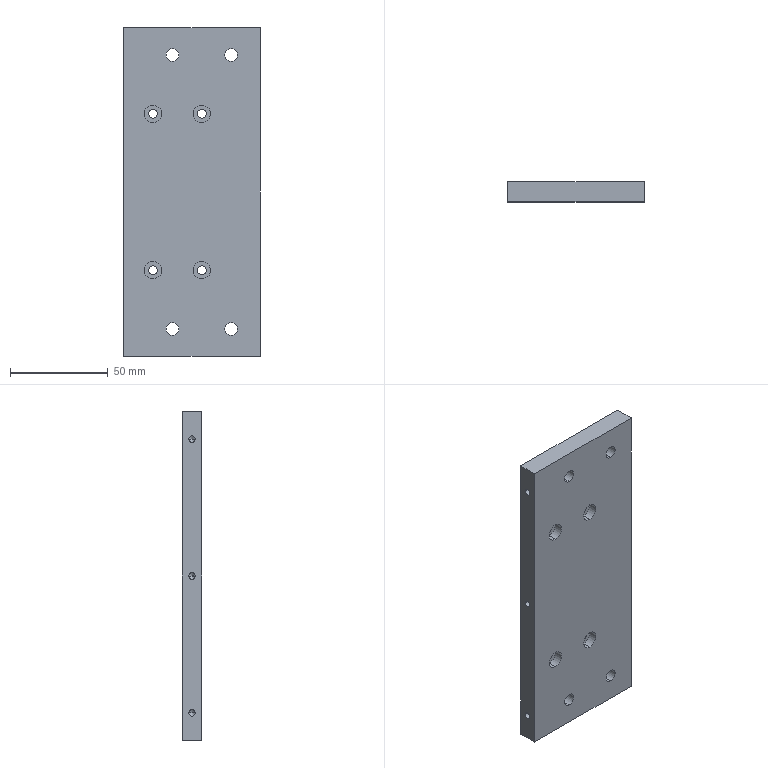Part | STEP file | 03-08 Support plate base | 1 solid | 46 faces | box 70 x 10 x 168 mm | volume 114407 mm3 | cylinder 30 | plane 10 | cone 6 | commonest cylinder face diameters 4.5 x8 6.5 x8 9 x8 3.3 x6